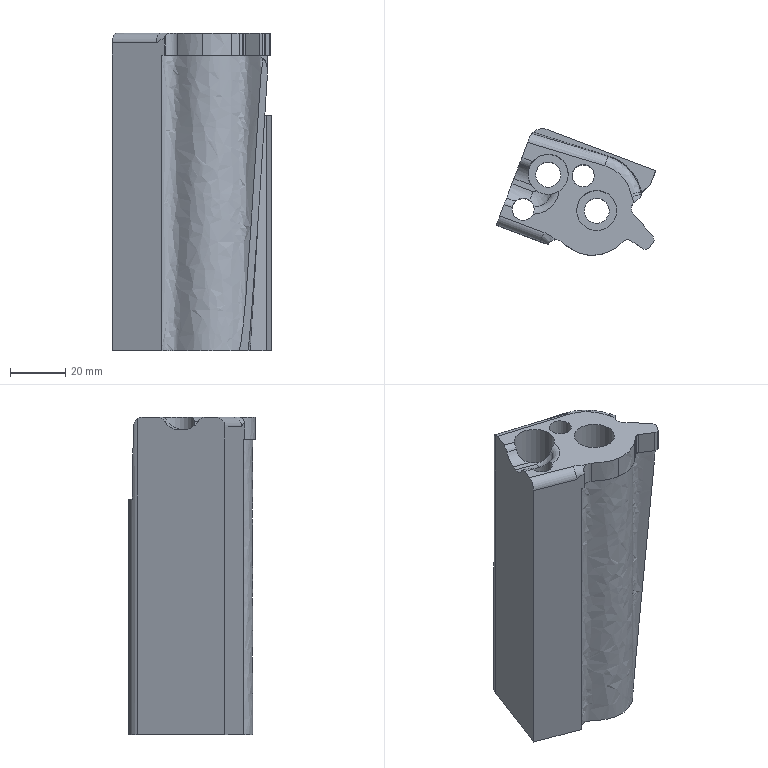Part | NX | features 23 2 | 1 solid | 63 faces | box 57.426 x 45.696 x 114.5 mm | volume 149195 mm3 | plane 23 | spline 20 | cylinder 18 | torus 2 | commonest cylinder face diameters 6 x4 4 x2 7 x2 8.001 x2 9 x2 13 x2